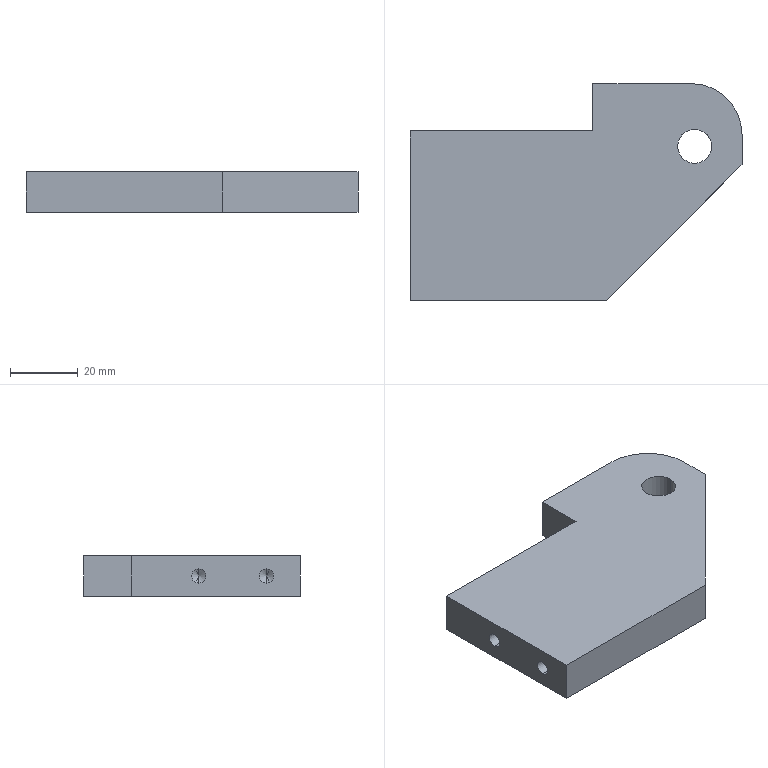Part | STEP file | PN_0032 Mount electronic clip wheel connecting mounting plate | 1 solid | 24 faces | box 98 x 64 x 12 mm | volume 54471 mm3 | cylinder 9 | plane 9 | cone 6 | commonest cylinder face diameters 4.2 x6 10 x2 30 x1